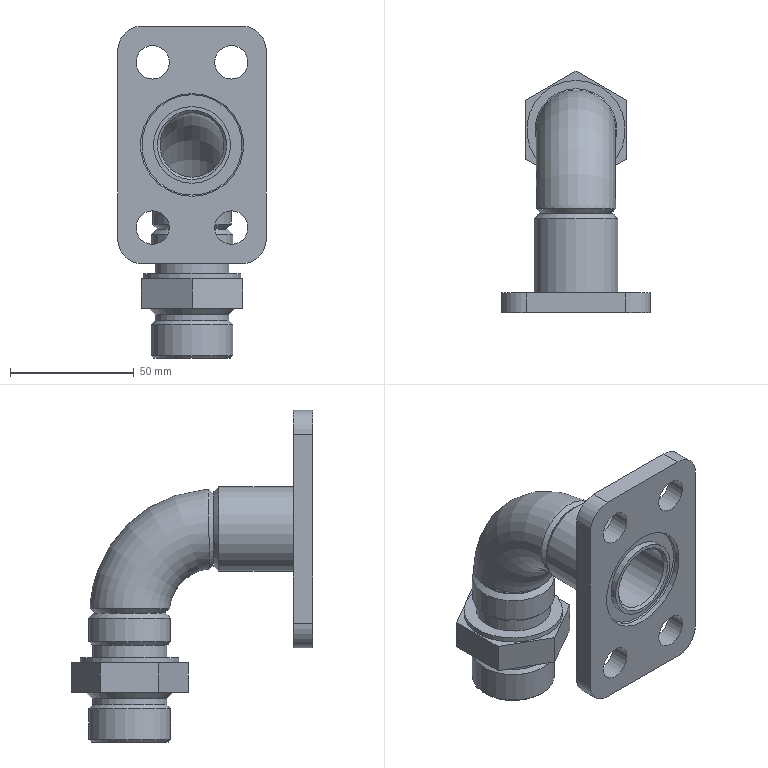Part | STEP file | HL4GZ-1.581.025 (variable pump outlet fitting weldment) | 4 solids | 56 faces | box 60 x 97.67 x 134 mm | volume 92965 mm3 | plane 23 | cylinder 19 | cone 9 | torus 3 | spline 2 | commonest cylinder face diameters 13.5 x4 20 x4 30 x2 31 x2 33 x2 21 x1